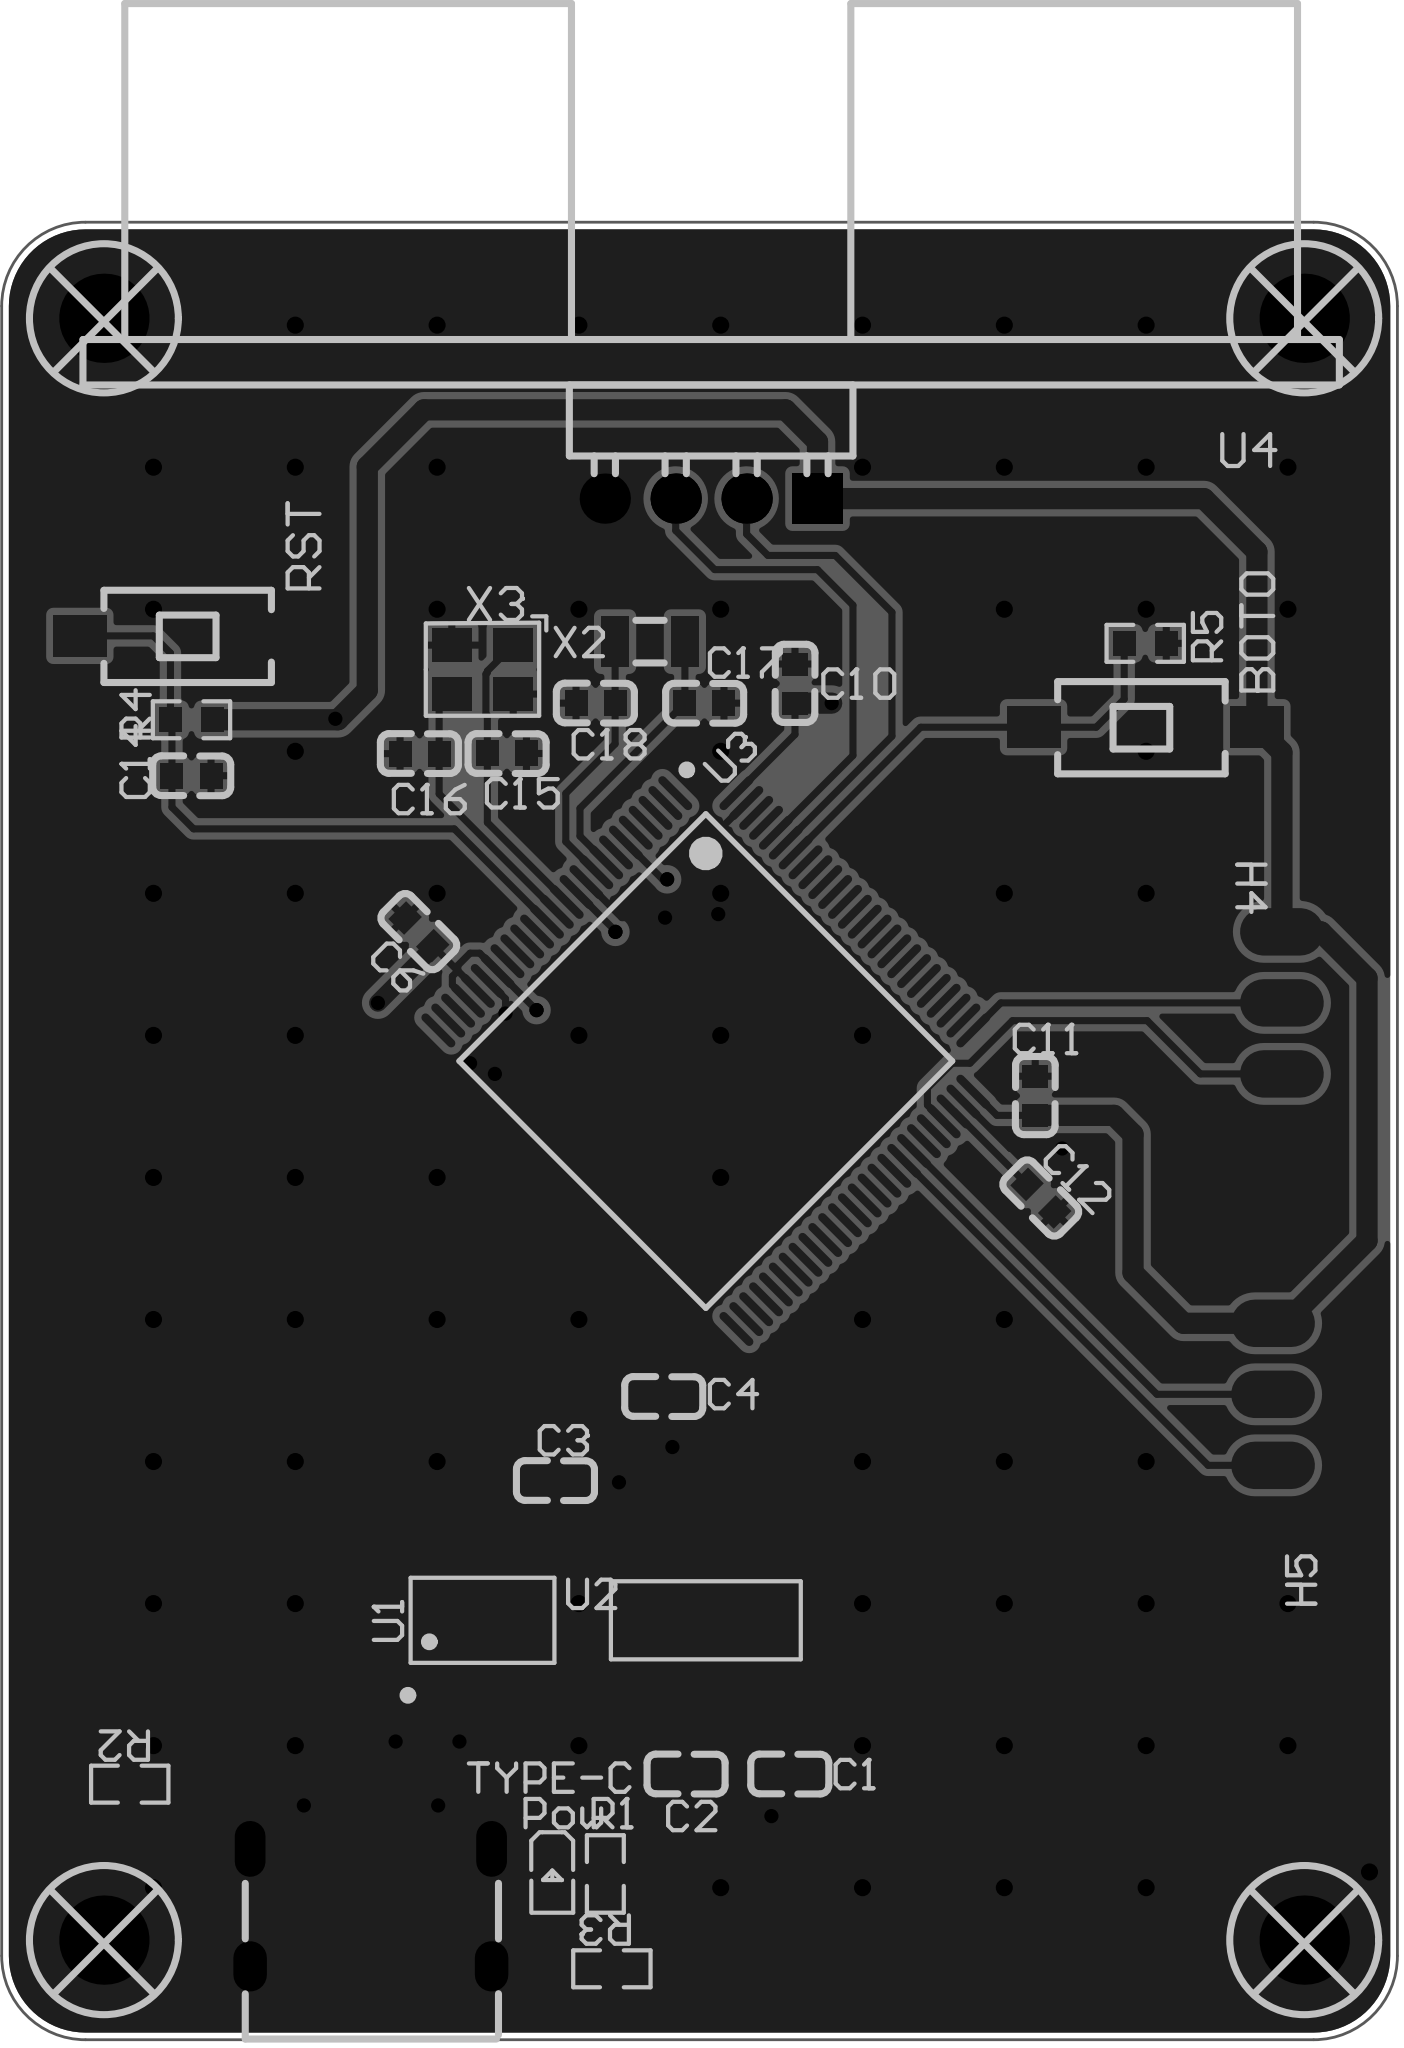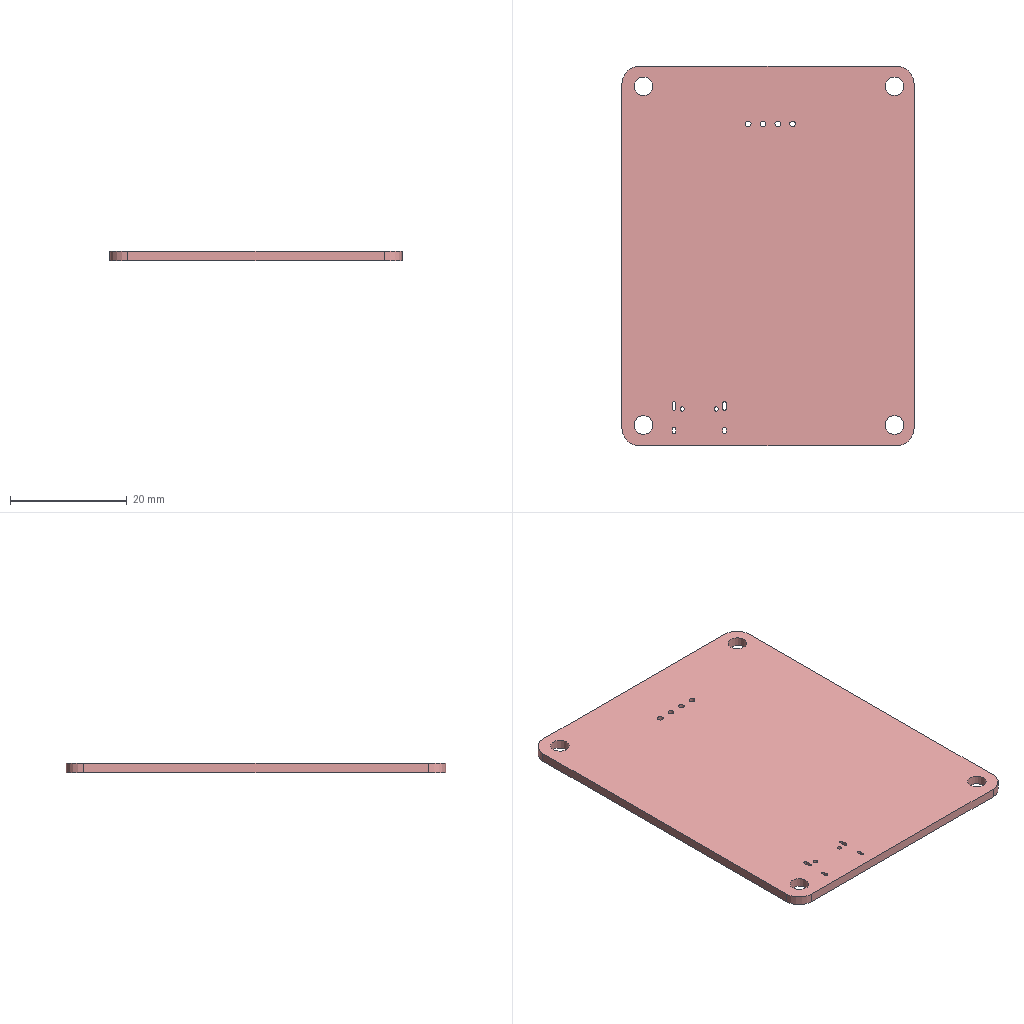Circuit board layout | Altium Designer | box 50 x 65 x 1.6 mm
Layer stack:
# Altium Designer layer stack of  (unit mm; dielectric type: 0 none, 1 core, 2 prepreg, 3 surface material)
index,name,kind,layer,copper_thickness_mm,dielectric_type,dielectric_thickness_mm,dielectric_material,dielectric_constant
0,Top Paste Mask Layer,other,,,,,,
1,Top Silkscreen Layer,other,,,,,,
2,Top Solder Mask Layer,dielectric,,,3,0.01,,3.3
3,Top Layer,copper,Top Layer,0.035,,,,
4,Dielectric1,dielectric,,,3,1.51,FR4,4.5
5,Bottom Layer,copper,Bottom Layer,0.035,,,,
6,Bottom Solder Mask Layer,dielectric,,,3,0.01,,3.3
7,Bottom Silkscreen Layer,other,,,,,,
8,Bottom Paste Mask Layer,other,,,,,,
# drill layer pairs: low layer,high layer
drill_pair,Top Layer,Bottom Layer
Part placement:
Designator,Comment,Layer,Footprint,Center-X(mm),Center-Y(mm),Rotation
X3,12MHz,TopLayer,OSC-SMD_4P-L3.2-W2.5-BL,114.873,136.252,180
C11,100nF,TopLayer,C0603,134.673,121.01,270
Pow,,TopLayer,LED_0603,117.365,93.184,270
C12,2.2uf,TopLayer,C0603,134.874,117.348,315
R1,1K,TopLayer,R0603,119.272,93.181,270
C4,100nF,TopLayer,C0603,121.373,110.252,0
TYPE-C,TYPE-C 16PIN 2MD(073),TopLayer,USB-C-SMD_TYPE-C-6PIN-2MD-073,110.873,92.252,0
R3,5.1K,TopLayer,R0603,119.507,89.789,180
R2,5.1K,TopLayer,R0603,102.235,96.393,0
U1,CH340N,TopLayer,SOP-8_L4.9-W3.9-P1.27-LS6.0-BL,114.873,102.252,0
C1,100nF,TopLayer,C0603,125.873,96.758,180
C10,100nF,TopLayer,C0603,126.067,135.752,270
C6,100nF,TopLayer,C0603,112.594,126.874,315
C3,100nF,TopLayer,C0603,117.478,107.252,180
C2,100nF,TopLayer,C0603,122.172,96.752,0
C18,12.5pF,TopLayer,C0603,118.922,135.052,0
C17,12.5pF,TopLayer,C0603,122.823,135.052,180
C16,20pF,TopLayer,C0603,112.618,133.247,0
C15,20pF,TopLayer,C0603,115.746,133.252,180
BOTO,TS-1101-C-W,TopLayer,SW-SMD_L6.0-W3.3-LS8.0,138.613,134.191,0
R4,10K,TopLayer,R0603,104.447,134.458,0
H5,,TopLayer,侧焊1X4排针,143.192,109.064,180
H4,,TopLayer,侧焊1X4排针,143.51,123.063,0
U3,,TopLayer,LQFP-100_L14.0-W14.0-P0.50-LS16.0-BL,122.873,122.252,225
X2,32.768kHz,TopLayer,FC-135R_L3.2-W1.5,120.873,137.252,180
R5,10K,TopLayer,R0603,138.613,137.191,180
C14,100nF,TopLayer,C0603,104.447,132.458,180
RST,TS-1101-C-W,TopLayer,SW-SMD_L6.0-W3.3-LS8.0,104.447,137.458,0
TP1,,TopLayer,M3螺丝,101.309,148.816,0
TP2,,TopLayer,M3螺丝,144.309,148.816,0
TP3,,TopLayer,M3螺丝,101.309,90.816,0
TP4,,TopLayer,M3螺丝,144.309,90.816,0
U2,LM1117IMPX-3.3/NOPB,TopLayer,SOT-223_L6.5-W3.5-P2.30-LS7.0-BR,122.873,102.252,270
U4,HC-SR04,TopLayer,TH_HC-SR04V,123.063,142.367,180
Pad and via stacks:
# Altium Designer via and pad stacks of  (unit mm). Each distinct definition once, with the count of objects using it.
# via: kind,start_layer,end_layer,hole_mm,diameter_mm,mode(0 simple;1 top-mid-bottom;2 full stack),diameter_per_layer,count,example_net
# pad: kind,layer,hole_mm,hole_type(0 round;1 square;2 slot),plating,top_size,top_shape(1 round;2 rect;3 octagon;9 rounded rect),mid_size,bottom_size,mode,footprint,size_per_layer,count,example
pad,Top Layer,0,0,plated,1.4x1.2,2,1.4x1.2,1.4x1.2,0,OSC-SMD_4P-L3.2-W2.5-BL,,4,X3.1
pad,Top Layer,0,0,plated,0.8x0.9,2,0.8x0.9,0.8x0.9,0,C0603,,26,C11.2
pad,Top Layer,0,0,plated,0.8001x0.8001,2,0.8001x0.8001,0.8001x0.8001,0,LED_0603,,2,Pow.1
pad,Top Layer,0,0,plated,0.8065x0.864,2,0.8065x0.864,0.8065x0.864,0,R0603,,10,R1.2
pad,Top Layer,0,0,plated,0.55x1.1,2,0.55x1.1,0.55x1.1,0,USB-C-SMD_TYPE-C-6PIN-2MD-073,,4,TYPE-C.1
pad,Top Layer,0,0,plated,0.3x1.1,2,0.3x1.1,0.3x1.1,0,USB-C-SMD_TYPE-C-6PIN-2MD-073,,8,TYPE-C.3
pad,Top Layer,0,0,plated,0.63x1.865,1,0.63x1.865,0.63x1.865,0,SOP-8_L4.9-W3.9-P1.27-LS6.0-BL,,8,U1.1
pad,Top Layer,0,0,plated,1.9x1.5,2,1.9x1.5,1.9x1.5,0,SW-SMD_L6.0-W3.3-LS8.0,,4,BOTO.1
pad,Top Layer,0,0,plated,3x1.7,1,3x1.7,3x1.7,0,\u00B2\u00E0\u00BA\u00B81X4\u00C5\u00C5\u00D5\u00EB,,8,H5.2
pad,Top Layer,0,0,plated,1.6x0.3,1,1.6x0.3,1.6x0.3,0,LQFP-100_L14.0-W14.0-P0.50-LS16.0-BL,,50,U3.100
pad,Top Layer,0,0,plated,0.3x1.6,1,0.3x1.6,0.3x1.6,0,LQFP-100_L14.0-W14.0-P0.50-LS16.0-BL,,50,U3.75
pad,Top Layer,0,0,plated,1.8x1,2,1.8x1,1.8x1,0,FC-135R_L3.2-W1.5,,2,X2.1
pad,Top Layer,0,0,plated,2.465x1.05,2,2.465x1.05,2.465x1.05,0,SOT-223_L6.5-W3.5-P2.30-LS7.0-BR,,3,U2.1
pad,Top Layer,0,0,plated,2.465x3.54,2,2.465x3.54,2.465x3.54,0,SOT-223_L6.5-W3.5-P2.30-LS7.0-BR,,1,U2.4
pad,Multi-Layer,0.6,2,plated,1.1x2,1,1.1x2,1.1x2,0,USB-C-SMD_TYPE-C-6PIN-2MD-073,,2,TYPE-C.13
pad,Multi-Layer,0.6,2,plated,1.2x1.8,1,1.2x1.8,1.2x1.8,0,USB-C-SMD_TYPE-C-6PIN-2MD-073,,2,TYPE-C.13
pad,Multi-Layer,3.2,0,plated,3.2x3.2,1,3.2x3.2,3.2x3.2,0,M3\u00C2\u00DD\u00CB\u00BF,,4,TP1.1
pad,Multi-Layer,1.001,0,plated,1.8x1.8,1,1.8x1.8,1.8x1.8,0,TH_HC-SR04V,,3,U4.4
pad,Multi-Layer,1.001,0,plated,1.8x1.8,2,1.8x1.8,1.8x1.8,0,TH_HC-SR04V,,1,U4.1
via,Top Layer,Bottom Layer,0.3048,0.6096,0,,1,GND
via,Top Layer,Bottom Layer,0.3048,0.508,0,,19,D-
via,Top Layer,Bottom Layer,0.3048,0.61,0,,70,GND
Copper pours:
name,layer,net,type(0 solid;1 hatched;2 none)
Top Layer-GND,Top Layer,GND,0
Bottom Layer-GND,Bottom Layer,GND,0
Design rules, without the lines most boards share:
# Altium Designer design rules of  (exported by Altium Designer, unit mm)
# columns: name | kind | enabled | priority | scope1 | scope2 | descriptor | typed fields (field=value)
Copper_copperRegion1 | 0 | disabled | 4 | All | All | Clearance Constraint (Gap=5.984mil) (Disabled)(All),(All) | gap=0.152
Copper_copperRegion1_1 | 63 | disabled | 4 | All | All | Board Clearance Constraint (Gap=0mil) (Disabled)(All) |
copperThickness1oz | 0 | enabled | 5 | All | All | Clearance Constraint (Gap=5.984mil) (All),(All) | gap=0.152
copperThickness1oz_1 | 63 | enabled | 5 | All | All | Board Clearance Constraint (Gap=0mil) (All) |
otherClearance | 52 | enabled | 1 | All | All | Hole To Hole Clearance (Gap=11.8mil) (All),(All) | gap=0.2997
differentialPair | 51 | enabled | 1 | All | All | Differential Pairs Uncoupled Length using the Gap Constraints (Min=6mil) (Max=10mil) (Prefered=10mil)  and Width Constraints (Min=5mil) (Max=100mil) (Prefered=10mil) (All) |
viaSize | 11 | enabled | 1 | All | All | Routing Via (MinHoleWidth=11.811mil) (MaxHoleWidth=247.992mil) (PreferredHoleWidth=12.008mil) (MinWidth=15.709mil) (MaxWidth=393.701mil) (PreferedWidth=24.016mil) (All) | via_min_hole=0.3 via_max_hole=6.299 via_preferred_diameter=0.61 via_preferred_hole=0.305
copperRegion1 | 20 | disabled | 1 | All | All | Polygon Connect Rule(Direct Connect )(Conductor Width=10mil) (Relief Angle=90 Angle) (Entries=4) (Air Gap Width=10mil) (Disabled)(All),(All) | connect_style(0=relief,1=direct,2=none)=1 relief_conductor_width=0.254 relief_entries=4
copperRegion | 20 | enabled | 2 | All | All | Polygon Connect Rule(Relief Connect )(Conductor Width=10mil) (Relief Angle=90 Angle) (Entries=4) (Air Gap Width=10mil) (All),(All) | connect_style(0=relief,1=direct,2=none)=0 relief_conductor_width=0.254 relief_entries=4
solderMaskExpansion | 13 | enabled | 2 | All | All | Solder Mask Expansion (Expansion =2.008mil) (All) | expansion=0.051